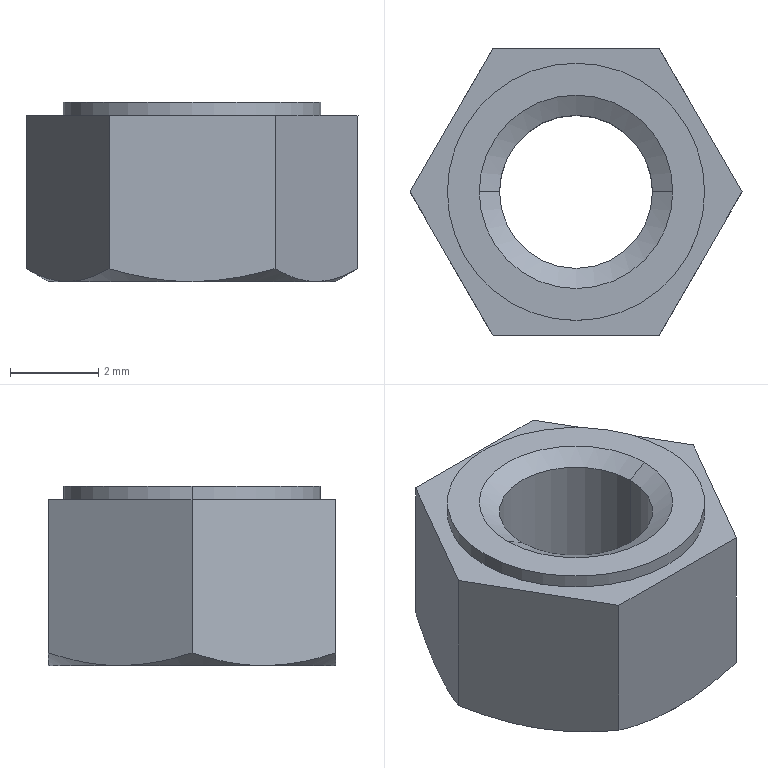Part | SolidWorks | features BaseBody 1, Scale 1 | 1 solid | 23 faces | box 7.506 x 6.5 x 4.05 mm | volume 105.396 mm3 | cone 10 | plane 9 | cylinder 4 | commonest cylinder face diameters 3.458 x2 5.815 x2
STEP:
#1=CARTESIAN_POINT('',(-1.729,0.000000001,-5.258));
#2=VERTEX_POINT('',#1);
#3=CARTESIAN_POINT('',(1.729,0.000000001,-5.258));
#4=VERTEX_POINT('',#3);
#5=CARTESIAN_POINT('',(0.000000001,0.000000001,-5.258));
#6=DIRECTION('',(0.,0.,1.));
#7=DIRECTION('',(1.,0.,0.));
#8=AXIS2_PLACEMENT_3D('',#5,#6,#7);
#9=CIRCLE('',#8,1.729);
#10=EDGE_CURVE('',#2,#4,#9,.T.);
#11=ORIENTED_EDGE('',*,*,#10,.F.);
#12=CARTESIAN_POINT('',(-1.729,0.000000001,-1.738));
#13=VERTEX_POINT('',#12);
#14=CARTESIAN_POINT('',(-1.729,0.000000001,-5.523));
#15=DIRECTION('',(0.,0.,1.));
#16=VECTOR('',#15,1000.);
#17=LINE('',#14,#16);
#18=EDGE_CURVE('',#2,#13,#17,.T.);
#19=ORIENTED_EDGE('',*,*,#18,.T.);
#20=CARTESIAN_POINT('',(1.729,0.000000001,-1.738));
#21=VERTEX_POINT('',#20);
#22=CARTESIAN_POINT('',(0.000000001,0.000000001,-1.738));
#23=DIRECTION('',(0.,0.,-1.));
#24=DIRECTION('',(1.,0.,0.));
#25=AXIS2_PLACEMENT_3D('',#22,#23,#24);
#26=CIRCLE('',#25,1.729);
#27=EDGE_CURVE('',#21,#13,#26,.T.);
#28=ORIENTED_EDGE('',*,*,#27,.F.);
#29=CARTESIAN_POINT('',(1.729,0.000000001,-5.523));
#30=DIRECTION('',(0.,0.,1.));
#31=VECTOR('',#30,1000.);
#32=LINE('',#29,#31);
#33=EDGE_CURVE('',#4,#21,#32,.T.);
#34=ORIENTED_EDGE('',*,*,#33,.F.);
#35=EDGE_LOOP('',(#11,#19,#28,#34));
#36=FACE_OUTER_BOUND('',#35,.T.);
#37=CARTESIAN_POINT('',(0.000000001,0.000000001,-5.523));
#38=DIRECTION('',(0.,0.,1.));
#39=DIRECTION('',(1.,0.,0.));
#40=AXIS2_PLACEMENT_3D('',#37,#38,#39);
#41=CYLINDRICAL_SURFACE('',#40,1.729);
#42=ADVANCED_FACE('',(#36),#41,.F.);
#43=ORIENTED_EDGE('',*,*,#10,.T.);
#44=CARTESIAN_POINT('',(2.188,0.000000001,-5.523));
#45=VERTEX_POINT('',#44);
#46=CARTESIAN_POINT('',(2.188,0.000000001,-5.523));
#47=DIRECTION('',(0.866,0.,-0.5));
#48=VECTOR('',#47,1000.);
#49=LINE('',#46,#48);
#50=EDGE_CURVE('',#4,#45,#49,.T.);
#51=ORIENTED_EDGE('',*,*,#50,.T.);
#52=CARTESIAN_POINT('',(-2.187,0.000000001,-5.523));
#53=VERTEX_POINT('',#52);
#54=CARTESIAN_POINT('',(0.000000001,0.000000001,-5.523));
#55=DIRECTION('',(0.,0.,1.));
#56=DIRECTION('',(-1.,0.,0.));
#57=AXIS2_PLACEMENT_3D('',#54,#55,#56);
#58=CIRCLE('',#57,2.187);
#59=EDGE_CURVE('',#53,#45,#58,.T.);
#60=ORIENTED_EDGE('',*,*,#59,.F.);
#61=CARTESIAN_POINT('',(-2.187,0.000000001,-5.523));
#62=DIRECTION('',(-0.866,0.,-0.5));
#63=VECTOR('',#62,1000.);
#64=LINE('',#61,#63);
#65=EDGE_CURVE('',#2,#53,#64,.T.);
#66=ORIENTED_EDGE('',*,*,#65,.F.);
#67=EDGE_LOOP('',(#43,#51,#60,#66));
#68=FACE_OUTER_BOUND('',#67,.T.);
#69=CARTESIAN_POINT('',(0.000000001,0.000000001,-5.523));
#70=DIRECTION('',(0.,0.,-1.));
#71=DIRECTION('',(-1.,0.,0.));
#72=AXIS2_PLACEMENT_3D('',#69,#70,#71);
#73=CONICAL_SURFACE('',#72,2.187,1.047);
#74=ADVANCED_FACE('',(#68),#73,.F.);
#75=ORIENTED_EDGE('',*,*,#27,.T.);
#76=CARTESIAN_POINT('',(-2.187,0.000000001,-1.473));
#77=VERTEX_POINT('',#76);
#78=CARTESIAN_POINT('',(-2.187,0.000000001,-1.473));
#79=DIRECTION('',(-0.866,0.,0.5));
#80=VECTOR('',#79,1000.);
#81=LINE('',#78,#80);
#82=EDGE_CURVE('',#13,#77,#81,.T.);
#83=ORIENTED_EDGE('',*,*,#82,.T.);
#84=CARTESIAN_POINT('',(2.188,0.000000001,-1.473));
#85=VERTEX_POINT('',#84);
#86=CARTESIAN_POINT('',(0.000000001,0.000000001,-1.473));
#87=DIRECTION('',(0.,0.,-1.));
#88=DIRECTION('',(1.,0.,0.));
#89=AXIS2_PLACEMENT_3D('',#86,#87,#88);
#90=CIRCLE('',#89,2.187);
#91=EDGE_CURVE('',#85,#77,#90,.T.);
#92=ORIENTED_EDGE('',*,*,#91,.F.);
#93=CARTESIAN_POINT('',(2.188,0.000000001,-1.473));
#94=DIRECTION('',(0.866,0.,0.5));
#95=VECTOR('',#94,1000.);
#96=LINE('',#93,#95);
#97=EDGE_CURVE('',#21,#85,#96,.T.);
#98=ORIENTED_EDGE('',*,*,#97,.F.);
#99=EDGE_LOOP('',(#75,#83,#92,#98));
#100=FACE_OUTER_BOUND('',#99,.T.);
#101=CARTESIAN_POINT('',(0.000000001,0.000000001,-1.473));
#102=DIRECTION('',(0.,0.,1.));
#103=DIRECTION('',(1.,0.,0.));
#104=AXIS2_PLACEMENT_3D('',#101,#102,#103);
#105=CONICAL_SURFACE('',#104,2.187,1.047);
#106=ADVANCED_FACE('',(#100),#105,.F.);
#107=CARTESIAN_POINT('',(2.908,0.000000001,-1.473));
#108=VERTEX_POINT('',#107);
#109=CARTESIAN_POINT('',(-2.907,0.000000001,-1.473));
#110=VERTEX_POINT('',#109);
#111=CARTESIAN_POINT('',(0.000000001,0.000000001,-1.473));
#112=DIRECTION('',(0.,0.,1.));
#113=DIRECTION('',(-1.,0.,0.));
#114=AXIS2_PLACEMENT_3D('',#111,#112,#113);
#115=CIRCLE('',#114,2.908);
#116=EDGE_CURVE('',#108,#110,#115,.T.);
#117=ORIENTED_EDGE('',*,*,#116,.F.);
#118=CARTESIAN_POINT('',(2.908,0.000000001,-1.773));
#119=VERTEX_POINT('',#118);
#120=CARTESIAN_POINT('',(2.908,0.000000001,-1.473));
#121=DIRECTION('',(0.,0.,-1.));
#122=VECTOR('',#121,1000.);
#123=LINE('',#120,#122);
#124=EDGE_CURVE('',#108,#119,#123,.T.);
#125=ORIENTED_EDGE('',*,*,#124,.T.);
#126=CARTESIAN_POINT('',(-2.907,0.000000001,-1.773));
#127=VERTEX_POINT('',#126);
#128=CARTESIAN_POINT('',(0.000000001,0.000000001,-1.773));
#129=DIRECTION('',(0.,0.,1.));
#130=DIRECTION('',(-1.,0.,0.));
#131=AXIS2_PLACEMENT_3D('',#128,#129,#130);
#132=CIRCLE('',#131,2.908);
#133=EDGE_CURVE('',#119,#127,#132,.T.);
#134=ORIENTED_EDGE('',*,*,#133,.T.);
#135=CARTESIAN_POINT('',(-2.907,0.000000001,-1.473));
#136=DIRECTION('',(0.,0.,-1.));
#137=VECTOR('',#136,1000.);
#138=LINE('',#135,#137);
#139=EDGE_CURVE('',#110,#127,#138,.T.);
#140=ORIENTED_EDGE('',*,*,#139,.F.);
#141=EDGE_LOOP('',(#117,#125,#134,#140));
#142=FACE_OUTER_BOUND('',#141,.T.);
#143=CARTESIAN_POINT('',(0.000000001,0.000000001,-1.473));
#144=DIRECTION('',(0.,0.,-1.));
#145=DIRECTION('',(-1.,0.,0.));
#146=AXIS2_PLACEMENT_3D('',#143,#144,#145);
#147=CYLINDRICAL_SURFACE('',#146,2.908);
#148=ADVANCED_FACE('',(#142),#147,.T.);
#149=ORIENTED_EDGE('',*,*,#18,.F.);
#150=CARTESIAN_POINT('',(0.000000001,0.000000001,-5.258));
#151=DIRECTION('',(0.,0.,1.));
#152=DIRECTION('',(1.,0.,0.));
#153=AXIS2_PLACEMENT_3D('',#150,#151,#152);
#154=CIRCLE('',#153,1.729);
#155=EDGE_CURVE('',#4,#2,#154,.T.);
#156=ORIENTED_EDGE('',*,*,#155,.F.);
#157=ORIENTED_EDGE('',*,*,#33,.T.);
#158=CARTESIAN_POINT('',(0.000000001,0.000000001,-1.738));
#159=DIRECTION('',(0.,0.,-1.));
#160=DIRECTION('',(1.,0.,0.));
#161=AXIS2_PLACEMENT_3D('',#158,#159,#160);
#162=CIRCLE('',#161,1.729);
#163=EDGE_CURVE('',#13,#21,#162,.T.);
#164=ORIENTED_EDGE('',*,*,#163,.F.);
#165=EDGE_LOOP('',(#149,#156,#157,#164));
#166=FACE_OUTER_BOUND('',#165,.T.);
#167=CARTESIAN_POINT('',(0.000000001,0.000000001,-5.523));
#168=DIRECTION('',(0.,0.,1.));
#169=DIRECTION('',(1.,0.,0.));
#170=AXIS2_PLACEMENT_3D('',#167,#168,#169);
#171=CYLINDRICAL_SURFACE('',#170,1.729);
#172=ADVANCED_FACE('',(#166),#171,.F.);
#173=ORIENTED_EDGE('',*,*,#50,.F.);
#174=ORIENTED_EDGE('',*,*,#155,.T.);
#175=ORIENTED_EDGE('',*,*,#65,.T.);
#176=CARTESIAN_POINT('',(0.000000001,0.000000001,-5.523));
#177=DIRECTION('',(0.,0.,1.));
#178=DIRECTION('',(-1.,0.,0.));
#179=AXIS2_PLACEMENT_3D('',#176,#177,#178);
#180=CIRCLE('',#179,2.187);
#181=EDGE_CURVE('',#45,#53,#180,.T.);
#182=ORIENTED_EDGE('',*,*,#181,.F.);
#183=EDGE_LOOP('',(#173,#174,#175,#182));
#184=FACE_OUTER_BOUND('',#183,.T.);
#185=CARTESIAN_POINT('',(0.000000001,0.000000001,-5.523));
#186=DIRECTION('',(0.,0.,-1.));
#187=DIRECTION('',(-1.,0.,0.));
#188=AXIS2_PLACEMENT_3D('',#185,#186,#187);
#189=CONICAL_SURFACE('',#188,2.187,1.047);
#190=ADVANCED_FACE('',(#184),#189,.F.);
#191=ORIENTED_EDGE('',*,*,#82,.F.);
#192=ORIENTED_EDGE('',*,*,#163,.T.);
#193=ORIENTED_EDGE('',*,*,#97,.T.);
#194=CARTESIAN_POINT('',(0.000000001,0.000000001,-1.473));
#195=DIRECTION('',(0.,0.,-1.));
#196=DIRECTION('',(1.,0.,0.));
#197=AXIS2_PLACEMENT_3D('',#194,#195,#196);
#198=CIRCLE('',#197,2.187);
#199=EDGE_CURVE('',#77,#85,#198,.T.);
#200=ORIENTED_EDGE('',*,*,#199,.F.);
#201=EDGE_LOOP('',(#191,#192,#193,#200));
#202=FACE_OUTER_BOUND('',#201,.T.);
#203=CARTESIAN_POINT('',(0.000000001,0.000000001,-1.473));
#204=DIRECTION('',(0.,0.,1.));
#205=DIRECTION('',(1.,0.,0.));
#206=AXIS2_PLACEMENT_3D('',#203,#204,#205);
#207=CONICAL_SURFACE('',#206,2.187,1.047);
#208=ADVANCED_FACE('',(#202),#207,.F.);
#209=CARTESIAN_POINT('',(2.815,-1.625,-5.523));
#210=VERTEX_POINT('',#209);
#211=CARTESIAN_POINT('',(2.815,1.625,-5.523));
#212=VERTEX_POINT('',#211);
#213=CARTESIAN_POINT('',(0.000000001,0.000000001,-5.523));
#214=DIRECTION('',(0.,0.,1.));
#215=DIRECTION('',(0.,-1.,0.));
#216=AXIS2_PLACEMENT_3D('',#213,#214,#215);
#217=CIRCLE('',#216,3.25);
#218=EDGE_CURVE('',#210,#212,#217,.T.);
#219=ORIENTED_EDGE('',*,*,#218,.F.);
#220=CARTESIAN_POINT('',(0.000000001,-3.25,-5.523));
#221=VERTEX_POINT('',#220);
#222=CARTESIAN_POINT('',(0.000000001,0.000000001,-5.523));
#223=DIRECTION('',(0.,0.,1.));
#224=DIRECTION('',(0.,-1.,0.));
#225=AXIS2_PLACEMENT_3D('',#222,#223,#224);
#226=CIRCLE('',#225,3.25);
#227=EDGE_CURVE('',#221,#210,#226,.T.);
#228=ORIENTED_EDGE('',*,*,#227,.F.);
#229=CARTESIAN_POINT('',(-2.815,-1.625,-5.523));
#230=VERTEX_POINT('',#229);
#231=CARTESIAN_POINT('',(0.000000001,0.000000001,-5.523));
#232=DIRECTION('',(0.,0.,1.));
#233=DIRECTION('',(0.,-1.,0.));
#234=AXIS2_PLACEMENT_3D('',#231,#232,#233);
#235=CIRCLE('',#234,3.25);
#236=EDGE_CURVE('',#230,#221,#235,.T.);
#237=ORIENTED_EDGE('',*,*,#236,.F.);
#238=CARTESIAN_POINT('',(-2.815,1.625,-5.523));
#239=VERTEX_POINT('',#238);
#240=CARTESIAN_POINT('',(0.000000001,0.000000001,-5.523));
#241=DIRECTION('',(0.,0.,1.));
#242=DIRECTION('',(0.,-1.,0.));
#243=AXIS2_PLACEMENT_3D('',#240,#241,#242);
#244=CIRCLE('',#243,3.25);
#245=EDGE_CURVE('',#239,#230,#244,.T.);
#246=ORIENTED_EDGE('',*,*,#245,.F.);
#247=CARTESIAN_POINT('',(0.000000001,3.25,-5.523));
#248=VERTEX_POINT('',#247);
#249=CARTESIAN_POINT('',(0.000000001,0.000000001,-5.523));
#250=DIRECTION('',(0.,0.,1.));
#251=DIRECTION('',(0.,-1.,0.));
#252=AXIS2_PLACEMENT_3D('',#249,#250,#251);
#253=CIRCLE('',#252,3.25);
#254=EDGE_CURVE('',#248,#239,#253,.T.);
#255=ORIENTED_EDGE('',*,*,#254,.F.);
#256=CARTESIAN_POINT('',(0.000000001,0.000000001,-5.523));
#257=DIRECTION('',(0.,0.,1.));
#258=DIRECTION('',(0.,-1.,0.));
#259=AXIS2_PLACEMENT_3D('',#256,#257,#258);
#260=CIRCLE('',#259,3.25);
#261=EDGE_CURVE('',#212,#248,#260,.T.);
#262=ORIENTED_EDGE('',*,*,#261,.F.);
#263=EDGE_LOOP('',(#219,#228,#237,#246,#255,#262));
#264=FACE_OUTER_BOUND('',#263,.T.);
#265=ORIENTED_EDGE('',*,*,#59,.T.);
#266=ORIENTED_EDGE('',*,*,#181,.T.);
#267=EDGE_LOOP('',(#265,#266));
#268=FACE_BOUND('',#267,.T.);
#269=CARTESIAN_POINT('',(5.629,-3.25,-5.523));
#270=DIRECTION('',(0.,0.,1.));
#271=DIRECTION('',(1.,0.,0.));
#272=AXIS2_PLACEMENT_3D('',#269,#270,#271);
#273=PLANE('',#272);
#274=ADVANCED_FACE('',(#264,#268),#273,.F.);
#275=CARTESIAN_POINT('',(0.000000001,0.000000001,-1.473));
#276=DIRECTION('',(0.,0.,1.));
#277=DIRECTION('',(-1.,0.,0.));
#278=AXIS2_PLACEMENT_3D('',#275,#276,#277);
#279=CIRCLE('',#278,2.908);
#280=EDGE_CURVE('',#110,#108,#279,.T.);
#281=ORIENTED_EDGE('',*,*,#280,.T.);
#282=ORIENTED_EDGE('',*,*,#116,.T.);
#283=EDGE_LOOP('',(#281,#282));
#284=FACE_OUTER_BOUND('',#283,.T.);
#285=ORIENTED_EDGE('',*,*,#91,.T.);
#286=ORIENTED_EDGE('',*,*,#199,.T.);
#287=EDGE_LOOP('',(#285,#286));
#288=FACE_BOUND('',#287,.T.);
#289=CARTESIAN_POINT('',(0.000000001,0.000000001,-1.473));
#290=DIRECTION('',(0.,0.,1.));
#291=DIRECTION('',(1.,0.,0.));
#292=AXIS2_PLACEMENT_3D('',#289,#290,#291);
#293=PLANE('',#292);
#294=ADVANCED_FACE('',(#284,#288),#293,.T.);
#295=ORIENTED_EDGE('',*,*,#261,.T.);
#296=CARTESIAN_POINT('',(1.876,3.25,-5.233));
#297=VERTEX_POINT('',#296);
#298=CARTESIAN_POINT('',(0.000000001,3.25,-5.523));
#299=CARTESIAN_POINT('',(0.6404,3.25,-5.523));
#300=CARTESIAN_POINT('',(1.263,3.25,-5.41));
#301=CARTESIAN_POINT('',(1.876,3.25,-5.233));
#302=B_SPLINE_CURVE_WITH_KNOTS('',3,(#298,#299,#300,#301),.UNSPECIFIED.,.F.,.F.,(4,4),(0.,0.001899),.UNSPECIFIED.);
#303=EDGE_CURVE('',#248,#297,#302,.T.);
#304=ORIENTED_EDGE('',*,*,#303,.T.);
#305=CARTESIAN_POINT('',(1.876,3.25,-5.233));
#306=CARTESIAN_POINT('',(2.183,2.719,-5.41));
#307=CARTESIAN_POINT('',(2.494,2.18,-5.523));
#308=CARTESIAN_POINT('',(2.815,1.625,-5.523));
#309=B_SPLINE_CURVE_WITH_KNOTS('',3,(#305,#306,#307,#308),.UNSPECIFIED.,.F.,.F.,(4,4),(0.,0.001899),.UNSPECIFIED.);
#310=EDGE_CURVE('',#297,#212,#309,.T.);
#311=ORIENTED_EDGE('',*,*,#310,.T.);
#312=EDGE_LOOP('',(#295,#304,#311));
#313=FACE_OUTER_BOUND('',#312,.T.);
#314=CARTESIAN_POINT('',(0.000000001,0.000000001,-5.231));
#315=DIRECTION('',(0.,0.,1.));
#316=DIRECTION('',(0.,-1.,0.));
#317=AXIS2_PLACEMENT_3D('',#314,#315,#316);
#318=CONICAL_SURFACE('',#317,3.756,1.047);
#319=ADVANCED_FACE('',(#313),#318,.T.);
#320=ORIENTED_EDGE('',*,*,#218,.T.);
#321=CARTESIAN_POINT('',(3.753,0.000000001,-5.233));
#322=VERTEX_POINT('',#321);
#323=CARTESIAN_POINT('',(2.815,1.625,-5.523));
#324=CARTESIAN_POINT('',(3.135,1.07,-5.523));
#325=CARTESIAN_POINT('',(3.446,0.5309,-5.41));
#326=CARTESIAN_POINT('',(3.753,0.000000001,-5.233));
#327=B_SPLINE_CURVE_WITH_KNOTS('',3,(#323,#324,#325,#326),.UNSPECIFIED.,.F.,.F.,(4,4),(0.,0.001899),.UNSPECIFIED.);
#328=EDGE_CURVE('',#212,#322,#327,.T.);
#329=ORIENTED_EDGE('',*,*,#328,.T.);
#330=CARTESIAN_POINT('',(3.753,0.000000001,-5.233));
#331=CARTESIAN_POINT('',(3.446,-0.5309,-5.41));
#332=CARTESIAN_POINT('',(3.135,-1.07,-5.523));
#333=CARTESIAN_POINT('',(2.815,-1.625,-5.523));
#334=B_SPLINE_CURVE_WITH_KNOTS('',3,(#330,#331,#332,#333),.UNSPECIFIED.,.F.,.F.,(4,4),(0.,0.001899),.UNSPECIFIED.);
#335=EDGE_CURVE('',#322,#210,#334,.T.);
#336=ORIENTED_EDGE('',*,*,#335,.T.);
#337=EDGE_LOOP('',(#320,#329,#336));
#338=FACE_OUTER_BOUND('',#337,.T.);
#339=CARTESIAN_POINT('',(0.000000001,0.000000001,-5.231));
#340=DIRECTION('',(0.,0.,1.));
#341=DIRECTION('',(0.,-1.,0.));
#342=AXIS2_PLACEMENT_3D('',#339,#340,#341);
#343=CONICAL_SURFACE('',#342,3.756,1.047);
#344=ADVANCED_FACE('',(#338),#343,.T.);
#345=CARTESIAN_POINT('',(1.876,-3.25,-5.233));
#346=VERTEX_POINT('',#345);
#347=CARTESIAN_POINT('',(2.815,-1.625,-5.523));
#348=CARTESIAN_POINT('',(2.494,-2.18,-5.523));
#349=CARTESIAN_POINT('',(2.183,-2.719,-5.41));
#350=CARTESIAN_POINT('',(1.876,-3.25,-5.233));
#351=B_SPLINE_CURVE_WITH_KNOTS('',3,(#347,#348,#349,#350),.UNSPECIFIED.,.F.,.F.,(4,4),(0.,0.001899),.UNSPECIFIED.);
#352=EDGE_CURVE('',#210,#346,#351,.T.);
#353=ORIENTED_EDGE('',*,*,#352,.T.);
#354=CARTESIAN_POINT('',(1.876,-3.25,-5.233));
#355=CARTESIAN_POINT('',(1.263,-3.25,-5.41));
#356=CARTESIAN_POINT('',(0.6404,-3.25,-5.523));
#357=CARTESIAN_POINT('',(0.000000001,-3.25,-5.523));
#358=B_SPLINE_CURVE_WITH_KNOTS('',3,(#354,#355,#356,#357),.UNSPECIFIED.,.F.,.F.,(4,4),(0.,0.001899),.UNSPECIFIED.);
#359=EDGE_CURVE('',#346,#221,#358,.T.);
#360=ORIENTED_EDGE('',*,*,#359,.T.);
#361=ORIENTED_EDGE('',*,*,#227,.T.);
#362=EDGE_LOOP('',(#353,#360,#361));
#363=FACE_OUTER_BOUND('',#362,.T.);
#364=CARTESIAN_POINT('',(0.000000001,0.000000001,-5.231));
#365=DIRECTION('',(0.,0.,1.));
#366=DIRECTION('',(0.,-1.,0.));
#367=AXIS2_PLACEMENT_3D('',#364,#365,#366);
#368=CONICAL_SURFACE('',#367,3.756,1.047);
#369=ADVANCED_FACE('',(#363),#368,.T.);
#370=CARTESIAN_POINT('',(-1.876,-3.25,-5.233));
#371=VERTEX_POINT('',#370);
#372=CARTESIAN_POINT('',(0.000000001,-3.25,-5.523));
#373=CARTESIAN_POINT('',(-0.6404,-3.25,-5.523));
#374=CARTESIAN_POINT('',(-1.263,-3.25,-5.41));
#375=CARTESIAN_POINT('',(-1.876,-3.25,-5.233));
#376=B_SPLINE_CURVE_WITH_KNOTS('',3,(#372,#373,#374,#375),.UNSPECIFIED.,.F.,.F.,(4,4),(0.,0.001899),.UNSPECIFIED.);
#377=EDGE_CURVE('',#221,#371,#376,.T.);
#378=ORIENTED_EDGE('',*,*,#377,.T.);
#379=CARTESIAN_POINT('',(-1.876,-3.25,-5.233));
#380=CARTESIAN_POINT('',(-2.183,-2.719,-5.41));
#381=CARTESIAN_POINT('',(-2.494,-2.18,-5.523));
#382=CARTESIAN_POINT('',(-2.815,-1.625,-5.523));
#383=B_SPLINE_CURVE_WITH_KNOTS('',3,(#379,#380,#381,#382),.UNSPECIFIED.,.F.,.F.,(4,4),(0.,0.001899),.UNSPECIFIED.);
#384=EDGE_CURVE('',#371,#230,#383,.T.);
#385=ORIENTED_EDGE('',*,*,#384,.T.);
#386=ORIENTED_EDGE('',*,*,#236,.T.);
#387=EDGE_LOOP('',(#378,#385,#386));
#388=FACE_OUTER_BOUND('',#387,.T.);
#389=CARTESIAN_POINT('',(0.000000001,0.000000001,-5.231));
#390=DIRECTION('',(0.,0.,1.));
#391=DIRECTION('',(0.,-1.,0.));
#392=AXIS2_PLACEMENT_3D('',#389,#390,#391);
#393=CONICAL_SURFACE('',#392,3.756,1.047);
#394=ADVANCED_FACE('',(#388),#393,.T.);
#395=CARTESIAN_POINT('',(-3.753,-0.000000017,-5.233));
#396=VERTEX_POINT('',#395);
#397=CARTESIAN_POINT('',(-2.815,-1.625,-5.523));
#398=CARTESIAN_POINT('',(-3.135,-1.07,-5.523));
#399=CARTESIAN_POINT('',(-3.446,-0.5309,-5.41));
#400=CARTESIAN_POINT('',(-3.753,-0.000000017,-5.233));
#401=B_SPLINE_CURVE_WITH_KNOTS('',3,(#397,#398,#399,#400),.UNSPECIFIED.,.F.,.F.,(4,4),(0.,0.001899),.UNSPECIFIED.);
#402=EDGE_CURVE('',#230,#396,#401,.T.);
#403=ORIENTED_EDGE('',*,*,#402,.T.);
#404=CARTESIAN_POINT('',(-3.753,-0.000000017,-5.233));
#405=CARTESIAN_POINT('',(-3.446,0.5309,-5.41));
#406=CARTESIAN_POINT('',(-3.135,1.07,-5.523));
#407=CARTESIAN_POINT('',(-2.815,1.625,-5.523));
#408=B_SPLINE_CURVE_WITH_KNOTS('',3,(#404,#405,#406,#407),.UNSPECIFIED.,.F.,.F.,(4,4),(0.,0.001899),.UNSPECIFIED.);
#409=EDGE_CURVE('',#396,#239,#408,.T.);
#410=ORIENTED_EDGE('',*,*,#409,.T.);
#411=ORIENTED_EDGE('',*,*,#245,.T.);
#412=EDGE_LOOP('',(#403,#410,#411));
#413=FACE_OUTER_BOUND('',#412,.T.);
#414=CARTESIAN_POINT('',(0.000000001,0.000000001,-5.231));
#415=DIRECTION('',(0.,0.,1.));
#416=DIRECTION('',(0.,-1.,0.));
#417=AXIS2_PLACEMENT_3D('',#414,#415,#416);
#418=CONICAL_SURFACE('',#417,3.756,1.047);
#419=ADVANCED_FACE('',(#413),#418,.T.);
#420=ORIENTED_EDGE('',*,*,#254,.T.);
#421=CARTESIAN_POINT('',(-1.876,3.25,-5.233));
#422=VERTEX_POINT('',#421);
#423=CARTESIAN_POINT('',(-2.815,1.625,-5.523));
#424=CARTESIAN_POINT('',(-2.494,2.18,-5.523));
#425=CARTESIAN_POINT('',(-2.183,2.719,-5.41));
#426=CARTESIAN_POINT('',(-1.876,3.25,-5.233));
#427=B_SPLINE_CURVE_WITH_KNOTS('',3,(#423,#424,#425,#426),.UNSPECIFIED.,.F.,.F.,(4,4),(0.,0.001899),.UNSPECIFIED.);
#428=EDGE_CURVE('',#239,#422,#427,.T.);
#429=ORIENTED_EDGE('',*,*,#428,.T.);
#430=CARTESIAN_POINT('',(-1.876,3.25,-5.233));
#431=CARTESIAN_POINT('',(-1.263,3.25,-5.41));
#432=CARTESIAN_POINT('',(-0.6404,3.25,-5.523));
#433=CARTESIAN_POINT('',(0.000000001,3.25,-5.523));
#434=B_SPLINE_CURVE_WITH_KNOTS('',3,(#430,#431,#432,#433),.UNSPECIFIED.,.F.,.F.,(4,4),(0.,0.001899),.UNSPECIFIED.);
#435=EDGE_CURVE('',#422,#248,#434,.T.);
#436=ORIENTED_EDGE('',*,*,#435,.T.);
#437=EDGE_LOOP('',(#420,#429,#436));
#438=FACE_OUTER_BOUND('',#437,.T.);
#439=CARTESIAN_POINT('',(0.000000001,0.000000001,-5.231));
#440=DIRECTION('',(0.,0.,1.));
#441=DIRECTION('',(0.,-1.,0.));
#442=AXIS2_PLACEMENT_3D('',#439,#440,#441);
#443=CONICAL_SURFACE('',#442,3.756,1.047);
#444=ADVANCED_FACE('',(#438),#443,.T.);
#445=ORIENTED_EDGE('',*,*,#124,.F.);
#446=ORIENTED_EDGE('',*,*,#280,.F.);
#447=ORIENTED_EDGE('',*,*,#139,.T.);
#448=CARTESIAN_POINT('',(0.000000001,0.000000001,-1.773));
#449=DIRECTION('',(0.,0.,1.));
#450=DIRECTION('',(-1.,0.,0.));
#451=AXIS2_PLACEMENT_3D('',#448,#449,#450);
#452=CIRCLE('',#451,2.908);
#453=EDGE_CURVE('',#127,#119,#452,.T.);
#454=ORIENTED_EDGE('',*,*,#453,.T.);
#455=EDGE_LOOP('',(#445,#446,#447,#454));
#456=FACE_OUTER_BOUND('',#455,.T.);
#457=CARTESIAN_POINT('',(0.000000001,0.000000001,-1.473));
#458=DIRECTION('',(0.,0.,-1.));
#459=DIRECTION('',(-1.,0.,0.));
#460=AXIS2_PLACEMENT_3D('',#457,#458,#459);
#461=CYLINDRICAL_SURFACE('',#460,2.908);
#462=ADVANCED_FACE('',(#456),#461,.T.);
#463=CARTESIAN_POINT('',(-1.876,3.25,-1.773));
#464=VERTEX_POINT('',#463);
#465=CARTESIAN_POINT('',(-1.876,3.25,-5.523));
#466=DIRECTION('',(0.,0.,1.));
#467=VECTOR('',#466,1000.);
#468=LINE('',#465,#467);
#469=EDGE_CURVE('',#422,#464,#468,.T.);
#470=ORIENTED_EDGE('',*,*,#469,.T.);
#471=CARTESIAN_POINT('',(1.876,3.25,-1.773));
#472=VERTEX_POINT('',#471);
#473=CARTESIAN_POINT('',(1.876,3.25,-1.773));
#474=DIRECTION('',(1.,0.,0.));
#475=VECTOR('',#474,1000.);
#476=LINE('',#473,#475);
#477=EDGE_CURVE('',#464,#472,#476,.T.);
#478=ORIENTED_EDGE('',*,*,#477,.T.);
#479=CARTESIAN_POINT('',(1.876,3.25,-5.523));
#480=DIRECTION('',(0.,0.,-1.));
#481=VECTOR('',#480,1000.);
#482=LINE('',#479,#481);
#483=EDGE_CURVE('',#472,#297,#482,.T.);
#484=ORIENTED_EDGE('',*,*,#483,.T.);
#485=ORIENTED_EDGE('',*,*,#303,.F.);
#486=ORIENTED_EDGE('',*,*,#435,.F.);
#487=EDGE_LOOP('',(#470,#478,#484,#485,#486));
#488=FACE_OUTER_BOUND('',#487,.T.);
#489=CARTESIAN_POINT('',(1.876,3.25,-5.523));
#490=DIRECTION('',(0.,1.,0.));
#491=DIRECTION('',(-1.,0.,0.));
#492=AXIS2_PLACEMENT_3D('',#489,#490,#491);
#493=PLANE('',#492);
#494=ADVANCED_FACE('',(#488),#493,.T.);
#495=ORIENTED_EDGE('',*,*,#483,.F.);
#496=CARTESIAN_POINT('',(3.753,0.000000001,-1.773));
#497=VERTEX_POINT('',#496);
#498=CARTESIAN_POINT('',(3.753,0.000000001,-1.773));
#499=DIRECTION('',(0.5,-0.866,0.));
#500=VECTOR('',#499,1000.);
#501=LINE('',#498,#500);
#502=EDGE_CURVE('',#472,#497,#501,.T.);
#503=ORIENTED_EDGE('',*,*,#502,.T.);
#504=CARTESIAN_POINT('',(3.753,0.000000001,-5.523));
#505=DIRECTION('',(0.,0.,-1.));
#506=VECTOR('',#505,1000.);
#507=LINE('',#504,#506);
#508=EDGE_CURVE('',#497,#322,#507,.T.);
#509=ORIENTED_EDGE('',*,*,#508,.T.);
#510=ORIENTED_EDGE('',*,*,#328,.F.);
#511=ORIENTED_EDGE('',*,*,#310,.F.);
#512=EDGE_LOOP('',(#495,#503,#509,#510,#511));
#513=FACE_OUTER_BOUND('',#512,.T.);
#514=CARTESIAN_POINT('',(3.753,0.000000001,-5.523));
#515=DIRECTION('',(0.866,0.5,0.));
#516=DIRECTION('',(-0.5,0.866,0.));
#517=AXIS2_PLACEMENT_3D('',#514,#515,#516);
#518=PLANE('',#517);
#519=ADVANCED_FACE('',(#513),#518,.T.);
#520=ORIENTED_EDGE('',*,*,#508,.F.);
#521=CARTESIAN_POINT('',(1.876,-3.25,-1.773));
#522=VERTEX_POINT('',#521);
#523=CARTESIAN_POINT('',(1.876,-3.25,-1.773));
#524=DIRECTION('',(-0.5,-0.866,0.));
#525=VECTOR('',#524,1000.);
#526=LINE('',#523,#525);
#527=EDGE_CURVE('',#497,#522,#526,.T.);
#528=ORIENTED_EDGE('',*,*,#527,.T.);
#529=CARTESIAN_POINT('',(1.876,-3.25,-5.523));
#530=DIRECTION('',(0.,0.,-1.));
#531=VECTOR('',#530,1000.);
#532=LINE('',#529,#531);
#533=EDGE_CURVE('',#522,#346,#532,.T.);
#534=ORIENTED_EDGE('',*,*,#533,.T.);
#535=ORIENTED_EDGE('',*,*,#352,.F.);
#536=ORIENTED_EDGE('',*,*,#335,.F.);
#537=EDGE_LOOP('',(#520,#528,#534,#535,#536));
#538=FACE_OUTER_BOUND('',#537,.T.);
#539=CARTESIAN_POINT('',(1.876,-3.25,-5.523));
#540=DIRECTION('',(0.866,-0.5,0.));
#541=DIRECTION('',(0.5,0.866,0.));
#542=AXIS2_PLACEMENT_3D('',#539,#540,#541);
#543=PLANE('',#542);
#544=ADVANCED_FACE('',(#538),#543,.T.);
#545=ORIENTED_EDGE('',*,*,#533,.F.);
#546=CARTESIAN_POINT('',(-1.876,-3.25,-1.773));
#547=VERTEX_POINT('',#546);
#548=CARTESIAN_POINT('',(-1.876,-3.25,-1.773));
#549=DIRECTION('',(-1.,0.,0.));
#550=VECTOR('',#549,1000.);
#551=LINE('',#548,#550);
#552=EDGE_CURVE('',#522,#547,#551,.T.);
#553=ORIENTED_EDGE('',*,*,#552,.T.);
#554=CARTESIAN_POINT('',(-1.876,-3.25,-5.523));
#555=DIRECTION('',(0.,0.,-1.));
#556=VECTOR('',#555,1000.);
#557=LINE('',#554,#556);
#558=EDGE_CURVE('',#547,#371,#557,.T.);
#559=ORIENTED_EDGE('',*,*,#558,.T.);
#560=ORIENTED_EDGE('',*,*,#377,.F.);
#561=ORIENTED_EDGE('',*,*,#359,.F.);
#562=EDGE_LOOP('',(#545,#553,#559,#560,#561));
#563=FACE_OUTER_BOUND('',#562,.T.);
#564=CARTESIAN_POINT('',(-1.876,-3.25,-5.523));
#565=DIRECTION('',(0.,-1.,0.));
#566=DIRECTION('',(0.,0.,-1.));
#567=AXIS2_PLACEMENT_3D('',#564,#565,#566);
#568=PLANE('',#567);
#569=ADVANCED_FACE('',(#563),#568,.T.);
#570=ORIENTED_EDGE('',*,*,#558,.F.);
#571=CARTESIAN_POINT('',(-3.753,0.000000001,-1.773));
#572=VERTEX_POINT('',#571);
#573=CARTESIAN_POINT('',(-3.753,0.000000001,-1.773));
#574=DIRECTION('',(-0.5,0.866,0.));
#575=VECTOR('',#574,1000.);
#576=LINE('',#573,#575);
#577=EDGE_CURVE('',#547,#572,#576,.T.);
#578=ORIENTED_EDGE('',*,*,#577,.T.);
#579=CARTESIAN_POINT('',(-3.753,0.000000001,-5.523));
#580=DIRECTION('',(0.,0.,-1.));
#581=VECTOR('',#580,1000.);
#582=LINE('',#579,#581);
#583=EDGE_CURVE('',#572,#396,#582,.T.);
#584=ORIENTED_EDGE('',*,*,#583,.T.);
#585=ORIENTED_EDGE('',*,*,#402,.F.);
#586=ORIENTED_EDGE('',*,*,#384,.F.);
#587=EDGE_LOOP('',(#570,#578,#584,#585,#586));
#588=FACE_OUTER_BOUND('',#587,.T.);
#589=CARTESIAN_POINT('',(-3.753,0.000000001,-5.523));
#590=DIRECTION('',(-0.866,-0.5,0.));
#591=DIRECTION('',(0.5,-0.866,0.));
#592=AXIS2_PLACEMENT_3D('',#589,#590,#591);
#593=PLANE('',#592);
#594=ADVANCED_FACE('',(#588),#593,.T.);
#595=ORIENTED_EDGE('',*,*,#583,.F.);
#596=CARTESIAN_POINT('',(-1.876,3.25,-1.773));
#597=DIRECTION('',(0.5,0.866,0.));
#598=VECTOR('',#597,1000.);
#599=LINE('',#596,#598);
#600=EDGE_CURVE('',#572,#464,#599,.T.);
#601=ORIENTED_EDGE('',*,*,#600,.T.);
#602=ORIENTED_EDGE('',*,*,#469,.F.);
#603=ORIENTED_EDGE('',*,*,#428,.F.);
#604=ORIENTED_EDGE('',*,*,#409,.F.);
#605=EDGE_LOOP('',(#595,#601,#602,#603,#604));
#606=FACE_OUTER_BOUND('',#605,.T.);
#607=CARTESIAN_POINT('',(-1.876,3.25,-5.523));
#608=DIRECTION('',(-0.866,0.5,0.));
#609=DIRECTION('',(-0.5,-0.866,0.));
#610=AXIS2_PLACEMENT_3D('',#607,#608,#609);
#611=PLANE('',#610);
#612=ADVANCED_FACE('',(#606),#611,.T.);
#613=ORIENTED_EDGE('',*,*,#453,.F.);
#614=ORIENTED_EDGE('',*,*,#133,.F.);
#615=EDGE_LOOP('',(#613,#614));
#616=FACE_BOUND('',#615,.T.);
#617=ORIENTED_EDGE('',*,*,#600,.F.);
#618=ORIENTED_EDGE('',*,*,#577,.F.);
#619=ORIENTED_EDGE('',*,*,#552,.F.);
#620=ORIENTED_EDGE('',*,*,#527,.F.);
#621=ORIENTED_EDGE('',*,*,#502,.F.);
#622=ORIENTED_EDGE('',*,*,#477,.F.);
#623=EDGE_LOOP('',(#617,#618,#619,#620,#621,#622));
#624=FACE_OUTER_BOUND('',#623,.T.);
#625=CARTESIAN_POINT('',(5.629,-3.25,-1.773));
#626=DIRECTION('',(0.,0.,1.));
#627=DIRECTION('',(1.,0.,0.));
#628=AXIS2_PLACEMENT_3D('',#625,#626,#627);
#629=PLANE('',#628);
#630=ADVANCED_FACE('',(#616,#624),#629,.T.);
#631=CLOSED_SHELL('',(#42,#74,#106,#148,#172,#190,#208,#274,#294,#319,#344,#369,#394,#419,#444,#462,#494,#519,#544,#569,#594,#612,#630));
#632=MANIFOLD_SOLID_BREP('',#631);
#633=CARTESIAN_POINT('',(0.,0.,0.));
#634=DIRECTION('',(0.,0.,1.));
#635=DIRECTION('',(1.,0.,0.));
#636=AXIS2_PLACEMENT_3D('',#633,#634,#635);
#637=(LENGTH_UNIT()NAMED_UNIT(*)SI_UNIT(.MILLI.,.METRE.));
#638=UNCERTAINTY_MEASURE_WITH_UNIT(LENGTH_MEASURE(0.00001),#637,'','');
#639=(NAMED_UNIT(*)PLANE_ANGLE_UNIT()SI_UNIT($,.RADIAN.));
#640=(NAMED_UNIT(*)SI_UNIT($,.STERADIAN.)SOLID_ANGLE_UNIT());
#641=(GEOMETRIC_REPRESENTATION_CONTEXT(3)GLOBAL_UNCERTAINTY_ASSIGNED_CONTEXT((#638))GLOBAL_UNIT_ASSIGNED_CONTEXT((#637,#639,#640))REPRESENTATION_CONTEXT('',''));
#642=ADVANCED_BREP_SHAPE_REPRESENTATION('',(#632,#636),#641);